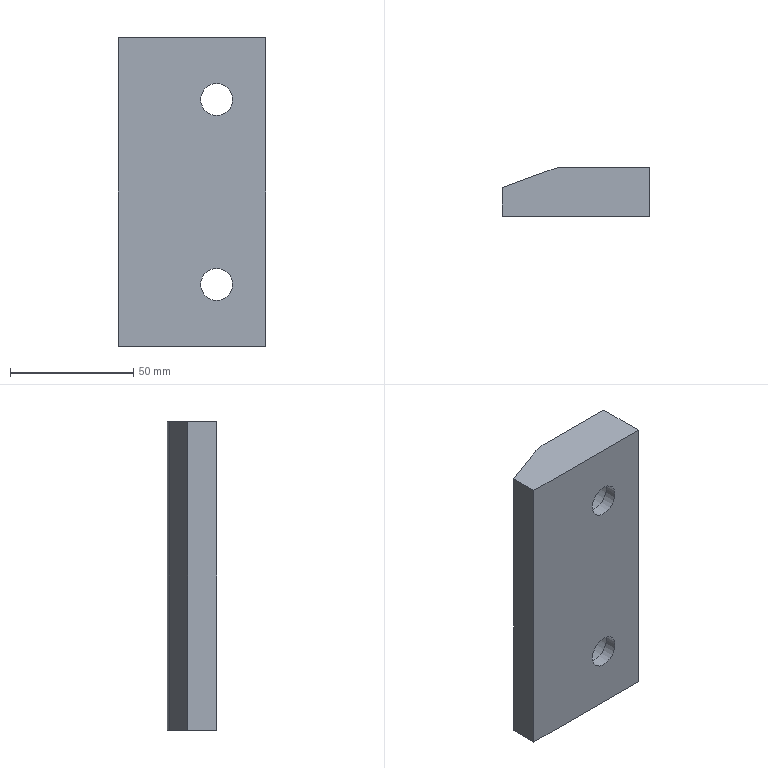Part | NX | features MAIN_BODY 2 | 1 solid | 14 faces | box 60 x 20 x 125 mm | volume 127417 mm3 | plane 9 | cylinder 5 | commonest cylinder face diameters 13 x2 20 x2 30 x1
STEP:
#1=CARTESIAN_POINT('',(254.,365.,-100.));
#2=VERTEX_POINT('',#1);
#3=CARTESIAN_POINT('',(254.,365.,-225.));
#4=VERTEX_POINT('',#3);
#5=CARTESIAN_POINT('',(254.,365.,-175.));
#6=DIRECTION('',(0.,0.,-1.));
#7=VECTOR('',#6,1000.);
#8=LINE('',#5,#7);
#9=EDGE_CURVE('',#2,#4,#8,.T.);
#10=ORIENTED_EDGE('',*,*,#9,.T.);
#11=CARTESIAN_POINT('',(314.,365.,-225.));
#12=VERTEX_POINT('',#11);
#13=CARTESIAN_POINT('',(229.,365.,-225.));
#14=DIRECTION('',(1.,0.,0.));
#15=VECTOR('',#14,1000.);
#16=LINE('',#13,#15);
#17=EDGE_CURVE('',#4,#12,#16,.T.);
#18=ORIENTED_EDGE('',*,*,#17,.T.);
#19=CARTESIAN_POINT('',(314.,365.,-100.));
#20=VERTEX_POINT('',#19);
#21=CARTESIAN_POINT('',(314.,365.,-175.));
#22=DIRECTION('',(0.,0.,1.));
#23=VECTOR('',#22,1000.);
#24=LINE('',#21,#23);
#25=EDGE_CURVE('',#12,#20,#24,.T.);
#26=ORIENTED_EDGE('',*,*,#25,.T.);
#27=CARTESIAN_POINT('',(229.,365.,-100.));
#28=DIRECTION('',(-1.,0.,0.));
#29=VECTOR('',#28,1000.);
#30=LINE('',#27,#29);
#31=EDGE_CURVE('',#20,#2,#30,.T.);
#32=ORIENTED_EDGE('',*,*,#31,.T.);
#33=EDGE_LOOP('',(#10,#18,#26,#32));
#34=FACE_BOUND('',#33,.T.);
#35=CARTESIAN_POINT('',(287.5,365.,-125.));
#36=VERTEX_POINT('',#35);
#37=CARTESIAN_POINT('',(294.,365.,-125.));
#38=DIRECTION('',(0.,1.,0.));
#39=DIRECTION('',(-1.,0.,0.));
#40=AXIS2_PLACEMENT_3D('',#37,#38,#39);
#41=CIRCLE('',#40,6.5);
#42=EDGE_CURVE('',#36,#36,#41,.T.);
#43=ORIENTED_EDGE('',*,*,#42,.T.);
#44=EDGE_LOOP('',(#43));
#45=FACE_BOUND('',#44,.T.);
#46=CARTESIAN_POINT('',(287.5,365.,-200.));
#47=VERTEX_POINT('',#46);
#48=CARTESIAN_POINT('',(294.,365.,-200.));
#49=DIRECTION('',(0.,1.,0.));
#50=DIRECTION('',(-1.,0.,0.));
#51=AXIS2_PLACEMENT_3D('',#48,#49,#50);
#52=CIRCLE('',#51,6.5);
#53=EDGE_CURVE('',#47,#47,#52,.T.);
#54=ORIENTED_EDGE('',*,*,#53,.T.);
#55=EDGE_LOOP('',(#54));
#56=FACE_BOUND('',#55,.T.);
#57=CARTESIAN_POINT('',(229.,365.,-175.));
#58=DIRECTION('',(0.,-1.,0.));
#59=DIRECTION('',(-1.,0.,0.));
#60=AXIS2_PLACEMENT_3D('',#57,#58,#59);
#61=PLANE('',#60);
#62=ADVANCED_FACE('',(#34,#45,#56),#61,.T.);
#63=CARTESIAN_POINT('',(314.,385.,-100.));
#64=VERTEX_POINT('',#63);
#65=CARTESIAN_POINT('',(314.,385.,-225.));
#66=VERTEX_POINT('',#65);
#67=CARTESIAN_POINT('',(314.,385.,-175.));
#68=DIRECTION('',(0.,0.,-1.));
#69=VECTOR('',#68,1000.);
#70=LINE('',#67,#69);
#71=EDGE_CURVE('',#64,#66,#70,.T.);
#72=ORIENTED_EDGE('',*,*,#71,.T.);
#73=CARTESIAN_POINT('',(279.402,385.,-225.));
#74=VERTEX_POINT('',#73);
#75=CARTESIAN_POINT('',(229.,385.,-225.));
#76=DIRECTION('',(-1.,0.,0.));
#77=VECTOR('',#76,1000.);
#78=LINE('',#75,#77);
#79=EDGE_CURVE('',#66,#74,#78,.T.);
#80=ORIENTED_EDGE('',*,*,#79,.T.);
#81=CARTESIAN_POINT('',(279.402,385.,-100.));
#82=VERTEX_POINT('',#81);
#83=CARTESIAN_POINT('',(279.402,385.,-175.));
#84=DIRECTION('',(0.,0.,1.));
#85=VECTOR('',#84,1000.);
#86=LINE('',#83,#85);
#87=EDGE_CURVE('',#74,#82,#86,.T.);
#88=ORIENTED_EDGE('',*,*,#87,.T.);
#89=CARTESIAN_POINT('',(379.,385.,-100.));
#90=DIRECTION('',(1.,0.,0.));
#91=VECTOR('',#90,1000.);
#92=LINE('',#89,#91);
#93=EDGE_CURVE('',#82,#64,#92,.T.);
#94=ORIENTED_EDGE('',*,*,#93,.T.);
#95=EDGE_LOOP('',(#72,#80,#88,#94));
#96=FACE_BOUND('',#95,.T.);
#97=CARTESIAN_POINT('',(294.,385.,-115.));
#98=VERTEX_POINT('',#97);
#99=CARTESIAN_POINT('',(294.,385.,-125.));
#100=DIRECTION('',(0.,-1.,0.));
#101=DIRECTION('',(0.,0.,1.));
#102=AXIS2_PLACEMENT_3D('',#99,#100,#101);
#103=CIRCLE('',#102,10.);
#104=EDGE_CURVE('',#98,#98,#103,.T.);
#105=ORIENTED_EDGE('',*,*,#104,.T.);
#106=EDGE_LOOP('',(#105));
#107=FACE_BOUND('',#106,.T.);
#108=CARTESIAN_POINT('',(294.,385.,-190.));
#109=VERTEX_POINT('',#108);
#110=CARTESIAN_POINT('',(294.,385.,-200.));
#111=DIRECTION('',(0.,-1.,0.));
#112=DIRECTION('',(0.,0.,1.));
#113=AXIS2_PLACEMENT_3D('',#110,#111,#112);
#114=CIRCLE('',#113,10.);
#115=EDGE_CURVE('',#109,#109,#114,.T.);
#116=ORIENTED_EDGE('',*,*,#115,.T.);
#117=EDGE_LOOP('',(#116));
#118=FACE_BOUND('',#117,.T.);
#119=CARTESIAN_POINT('',(379.,385.,-175.));
#120=DIRECTION('',(0.,1.,0.));
#121=DIRECTION('',(0.,0.,1.));
#122=AXIS2_PLACEMENT_3D('',#119,#120,#121);
#123=PLANE('',#122);
#124=ADVANCED_FACE('',(#96,#107,#118),#123,.T.);
#125=CARTESIAN_POINT('',(274.271,384.095,-100.));
#126=VERTEX_POINT('',#125);
#127=CARTESIAN_POINT('',(274.271,384.095,-225.));
#128=VERTEX_POINT('',#127);
#129=CARTESIAN_POINT('',(274.271,384.095,-175.));
#130=DIRECTION('',(0.,0.,1.));
#131=VECTOR('',#130,1000.);
#132=LINE('',#129,#131);
#133=EDGE_CURVE('',#126,#128,#132,.F.);
#134=ORIENTED_EDGE('',*,*,#133,.T.);
#135=CARTESIAN_POINT('',(254.,376.717,-225.));
#136=VERTEX_POINT('',#135);
#137=CARTESIAN_POINT('',(242.382,372.489,-225.));
#138=DIRECTION('',(-0.9397,-0.342,0.));
#139=VECTOR('',#138,1000.);
#140=LINE('',#137,#139);
#141=EDGE_CURVE('',#128,#136,#140,.T.);
#142=ORIENTED_EDGE('',*,*,#141,.T.);
#143=CARTESIAN_POINT('',(254.,376.717,-100.));
#144=VERTEX_POINT('',#143);
#145=CARTESIAN_POINT('',(254.,376.717,-175.));
#146=DIRECTION('',(0.,0.,1.));
#147=VECTOR('',#146,1000.);
#148=LINE('',#145,#147);
#149=EDGE_CURVE('',#136,#144,#148,.T.);
#150=ORIENTED_EDGE('',*,*,#149,.T.);
#151=CARTESIAN_POINT('',(291.21,390.261,-100.));
#152=DIRECTION('',(0.9397,0.342,0.));
#153=VECTOR('',#152,1000.);
#154=LINE('',#151,#153);
#155=EDGE_CURVE('',#144,#126,#154,.T.);
#156=ORIENTED_EDGE('',*,*,#155,.T.);
#157=EDGE_LOOP('',(#134,#142,#150,#156));
#158=FACE_BOUND('',#157,.T.);
#159=CARTESIAN_POINT('',(291.21,390.261,-175.));
#160=DIRECTION('',(-0.342,0.9397,0.));
#161=DIRECTION('',(0.9397,0.342,0.));
#162=AXIS2_PLACEMENT_3D('',#159,#160,#161);
#163=PLANE('',#162);
#164=ADVANCED_FACE('',(#158),#163,.T.);
#165=CARTESIAN_POINT('',(254.,395.,-100.));
#166=DIRECTION('',(0.,1.,0.));
#167=VECTOR('',#166,1000.);
#168=LINE('',#165,#167);
#169=EDGE_CURVE('',#2,#144,#168,.T.);
#170=ORIENTED_EDGE('',*,*,#169,.T.);
#171=ORIENTED_EDGE('',*,*,#149,.F.);
#172=CARTESIAN_POINT('',(254.,360.359,-225.));
#173=DIRECTION('',(0.,-1.,0.));
#174=VECTOR('',#173,1000.);
#175=LINE('',#172,#174);
#176=EDGE_CURVE('',#136,#4,#175,.T.);
#177=ORIENTED_EDGE('',*,*,#176,.T.);
#178=ORIENTED_EDGE('',*,*,#9,.F.);
#179=EDGE_LOOP('',(#170,#171,#177,#178));
#180=FACE_BOUND('',#179,.T.);
#181=CARTESIAN_POINT('',(254.,360.359,-175.));
#182=DIRECTION('',(-1.,0.,0.));
#183=DIRECTION('',(0.,0.,-1.));
#184=AXIS2_PLACEMENT_3D('',#181,#182,#183);
#185=PLANE('',#184);
#186=ADVANCED_FACE('',(#180),#185,.T.);
#187=CARTESIAN_POINT('',(314.,395.,-100.));
#188=DIRECTION('',(0.,1.,0.));
#189=VECTOR('',#188,1000.);
#190=LINE('',#187,#189);
#191=EDGE_CURVE('',#20,#64,#190,.T.);
#192=ORIENTED_EDGE('',*,*,#191,.F.);
#193=ORIENTED_EDGE('',*,*,#25,.F.);
#194=CARTESIAN_POINT('',(314.,395.,-225.));
#195=DIRECTION('',(0.,1.,0.));
#196=VECTOR('',#195,1000.);
#197=LINE('',#194,#196);
#198=EDGE_CURVE('',#12,#66,#197,.T.);
#199=ORIENTED_EDGE('',*,*,#198,.T.);
#200=ORIENTED_EDGE('',*,*,#71,.F.);
#201=EDGE_LOOP('',(#192,#193,#199,#200));
#202=FACE_BOUND('',#201,.T.);
#203=CARTESIAN_POINT('',(314.,350.,-175.));
#204=DIRECTION('',(1.,0.,0.));
#205=DIRECTION('',(0.,0.,1.));
#206=AXIS2_PLACEMENT_3D('',#203,#204,#205);
#207=PLANE('',#206);
#208=ADVANCED_FACE('',(#202),#207,.T.);
#209=ORIENTED_EDGE('',*,*,#93,.F.);
#210=CARTESIAN_POINT('',(279.402,370.,-100.));
#211=DIRECTION('',(0.,0.,-1.));
#212=DIRECTION('',(1.,0.,0.));
#213=AXIS2_PLACEMENT_3D('',#210,#211,#212);
#214=CIRCLE('',#213,15.);
#215=EDGE_CURVE('',#82,#126,#214,.F.);
#216=ORIENTED_EDGE('',*,*,#215,.T.);
#217=ORIENTED_EDGE('',*,*,#155,.F.);
#218=ORIENTED_EDGE('',*,*,#169,.F.);
#219=ORIENTED_EDGE('',*,*,#31,.F.);
#220=ORIENTED_EDGE('',*,*,#191,.T.);
#221=EDGE_LOOP('',(#209,#216,#217,#218,#219,#220));
#222=FACE_BOUND('',#221,.T.);
#223=CARTESIAN_POINT('',(229.,395.,-100.));
#224=DIRECTION('',(0.,0.,-1.));
#225=DIRECTION('',(1.,0.,0.));
#226=AXIS2_PLACEMENT_3D('',#223,#224,#225);
#227=PLANE('',#226);
#228=ADVANCED_FACE('',(#222),#227,.F.);
#229=ORIENTED_EDGE('',*,*,#42,.F.);
#230=EDGE_LOOP('',(#229));
#231=FACE_BOUND('',#230,.T.);
#232=CARTESIAN_POINT('',(287.5,370.,-125.));
#233=VERTEX_POINT('',#232);
#234=CARTESIAN_POINT('',(294.,370.,-125.));
#235=DIRECTION('',(0.,1.,0.));
#236=DIRECTION('',(-1.,0.,0.));
#237=AXIS2_PLACEMENT_3D('',#234,#235,#236);
#238=CIRCLE('',#237,6.5);
#239=EDGE_CURVE('',#233,#233,#238,.T.);
#240=ORIENTED_EDGE('',*,*,#239,.T.);
#241=EDGE_LOOP('',(#240));
#242=FACE_BOUND('',#241,.T.);
#243=CARTESIAN_POINT('',(294.,350.,-125.));
#244=DIRECTION('',(0.,-1.,0.));
#245=DIRECTION('',(0.,0.,-1.));
#246=AXIS2_PLACEMENT_3D('',#243,#244,#245);
#247=CYLINDRICAL_SURFACE('',#246,6.5);
#248=ADVANCED_FACE('',(#231,#242),#247,.F.);
#249=ORIENTED_EDGE('',*,*,#239,.F.);
#250=EDGE_LOOP('',(#249));
#251=FACE_BOUND('',#250,.T.);
#252=CARTESIAN_POINT('',(284.,370.,-125.));
#253=VERTEX_POINT('',#252);
#254=CARTESIAN_POINT('',(294.,370.,-125.));
#255=DIRECTION('',(0.,1.,0.));
#256=DIRECTION('',(-1.,0.,0.));
#257=AXIS2_PLACEMENT_3D('',#254,#255,#256);
#258=CIRCLE('',#257,10.);
#259=EDGE_CURVE('',#253,#253,#258,.T.);
#260=ORIENTED_EDGE('',*,*,#259,.T.);
#261=EDGE_LOOP('',(#260));
#262=FACE_BOUND('',#261,.T.);
#263=CARTESIAN_POINT('',(319.,370.,-180.));
#264=DIRECTION('',(0.,-1.,0.));
#265=DIRECTION('',(0.,0.,-1.));
#266=AXIS2_PLACEMENT_3D('',#263,#264,#265);
#267=PLANE('',#266);
#268=ADVANCED_FACE('',(#251,#262),#267,.F.);
#269=ORIENTED_EDGE('',*,*,#104,.F.);
#270=EDGE_LOOP('',(#269));
#271=FACE_BOUND('',#270,.T.);
#272=ORIENTED_EDGE('',*,*,#259,.F.);
#273=EDGE_LOOP('',(#272));
#274=FACE_BOUND('',#273,.T.);
#275=CARTESIAN_POINT('',(294.,395.,-125.));
#276=DIRECTION('',(0.,-1.,0.));
#277=DIRECTION('',(0.,0.,-1.));
#278=AXIS2_PLACEMENT_3D('',#275,#276,#277);
#279=CYLINDRICAL_SURFACE('',#278,10.);
#280=ADVANCED_FACE('',(#271,#274),#279,.F.);
#281=ORIENTED_EDGE('',*,*,#215,.F.);
#282=ORIENTED_EDGE('',*,*,#87,.F.);
#283=CARTESIAN_POINT('',(279.402,370.,-225.));
#284=DIRECTION('',(0.,0.,-1.));
#285=DIRECTION('',(1.,0.,0.));
#286=AXIS2_PLACEMENT_3D('',#283,#284,#285);
#287=CIRCLE('',#286,15.);
#288=EDGE_CURVE('',#128,#74,#287,.T.);
#289=ORIENTED_EDGE('',*,*,#288,.F.);
#290=ORIENTED_EDGE('',*,*,#133,.F.);
#291=EDGE_LOOP('',(#281,#282,#289,#290));
#292=FACE_BOUND('',#291,.T.);
#293=CARTESIAN_POINT('',(279.402,370.,-175.));
#294=DIRECTION('',(0.,0.,1.));
#295=DIRECTION('',(-1.,0.,0.));
#296=AXIS2_PLACEMENT_3D('',#293,#294,#295);
#297=CYLINDRICAL_SURFACE('',#296,15.);
#298=ADVANCED_FACE('',(#292),#297,.T.);
#299=CARTESIAN_POINT('',(287.5,370.,-200.));
#300=VERTEX_POINT('',#299);
#301=CARTESIAN_POINT('',(294.,370.,-200.));
#302=DIRECTION('',(0.,1.,0.));
#303=DIRECTION('',(-1.,0.,0.));
#304=AXIS2_PLACEMENT_3D('',#301,#302,#303);
#305=CIRCLE('',#304,6.5);
#306=EDGE_CURVE('',#300,#300,#305,.T.);
#307=ORIENTED_EDGE('',*,*,#306,.F.);
#308=EDGE_LOOP('',(#307));
#309=FACE_BOUND('',#308,.T.);
#310=CARTESIAN_POINT('',(284.,370.,-200.));
#311=VERTEX_POINT('',#310);
#312=CARTESIAN_POINT('',(294.,370.,-200.));
#313=DIRECTION('',(0.,1.,0.));
#314=DIRECTION('',(-1.,0.,0.));
#315=AXIS2_PLACEMENT_3D('',#312,#313,#314);
#316=CIRCLE('',#315,10.);
#317=EDGE_CURVE('',#311,#311,#316,.T.);
#318=ORIENTED_EDGE('',*,*,#317,.T.);
#319=EDGE_LOOP('',(#318));
#320=FACE_BOUND('',#319,.T.);
#321=CARTESIAN_POINT('',(319.,370.,-230.));
#322=DIRECTION('',(0.,-1.,0.));
#323=DIRECTION('',(0.,0.,-1.));
#324=AXIS2_PLACEMENT_3D('',#321,#322,#323);
#325=PLANE('',#324);
#326=ADVANCED_FACE('',(#309,#320),#325,.F.);
#327=ORIENTED_EDGE('',*,*,#53,.F.);
#328=EDGE_LOOP('',(#327));
#329=FACE_BOUND('',#328,.T.);
#330=ORIENTED_EDGE('',*,*,#306,.T.);
#331=EDGE_LOOP('',(#330));
#332=FACE_BOUND('',#331,.T.);
#333=CARTESIAN_POINT('',(294.,350.,-200.));
#334=DIRECTION('',(0.,-1.,0.));
#335=DIRECTION('',(0.,0.,-1.));
#336=AXIS2_PLACEMENT_3D('',#333,#334,#335);
#337=CYLINDRICAL_SURFACE('',#336,6.5);
#338=ADVANCED_FACE('',(#329,#332),#337,.F.);
#339=ORIENTED_EDGE('',*,*,#115,.F.);
#340=EDGE_LOOP('',(#339));
#341=FACE_BOUND('',#340,.T.);
#342=ORIENTED_EDGE('',*,*,#317,.F.);
#343=EDGE_LOOP('',(#342));
#344=FACE_BOUND('',#343,.T.);
#345=CARTESIAN_POINT('',(294.,395.,-200.));
#346=DIRECTION('',(0.,-1.,0.));
#347=DIRECTION('',(0.,0.,-1.));
#348=AXIS2_PLACEMENT_3D('',#345,#346,#347);
#349=CYLINDRICAL_SURFACE('',#348,10.);
#350=ADVANCED_FACE('',(#341,#344),#349,.F.);
#351=ORIENTED_EDGE('',*,*,#141,.F.);
#352=ORIENTED_EDGE('',*,*,#288,.T.);
#353=ORIENTED_EDGE('',*,*,#79,.F.);
#354=ORIENTED_EDGE('',*,*,#198,.F.);
#355=ORIENTED_EDGE('',*,*,#17,.F.);
#356=ORIENTED_EDGE('',*,*,#176,.F.);
#357=EDGE_LOOP('',(#351,#352,#353,#354,#355,#356));
#358=FACE_BOUND('',#357,.T.);
#359=CARTESIAN_POINT('',(229.,395.,-225.));
#360=DIRECTION('',(0.,0.,-1.));
#361=DIRECTION('',(1.,0.,0.));
#362=AXIS2_PLACEMENT_3D('',#359,#360,#361);
#363=PLANE('',#362);
#364=ADVANCED_FACE('',(#358),#363,.T.);
#365=CLOSED_SHELL('',(#62,#124,#164,#186,#208,#228,#248,#268,#280,#298,#326,#338,#350,#364));
#366=MANIFOLD_SOLID_BREP('',#365);
#367=(LENGTH_UNIT()NAMED_UNIT(*)SI_UNIT(.MILLI.,.METRE.));
#368=UNCERTAINTY_MEASURE_WITH_UNIT(LENGTH_MEASURE(0.00001),#367,'','');
#369=(NAMED_UNIT(*)PLANE_ANGLE_UNIT()SI_UNIT($,.RADIAN.));
#370=(NAMED_UNIT(*)SI_UNIT($,.STERADIAN.)SOLID_ANGLE_UNIT());
#371=(GEOMETRIC_REPRESENTATION_CONTEXT(3)GLOBAL_UNCERTAINTY_ASSIGNED_CONTEXT((#368))GLOBAL_UNIT_ASSIGNED_CONTEXT((#367,#369,#370))REPRESENTATION_CONTEXT('',''));
#372=ADVANCED_BREP_SHAPE_REPRESENTATION('',(#366),#371);